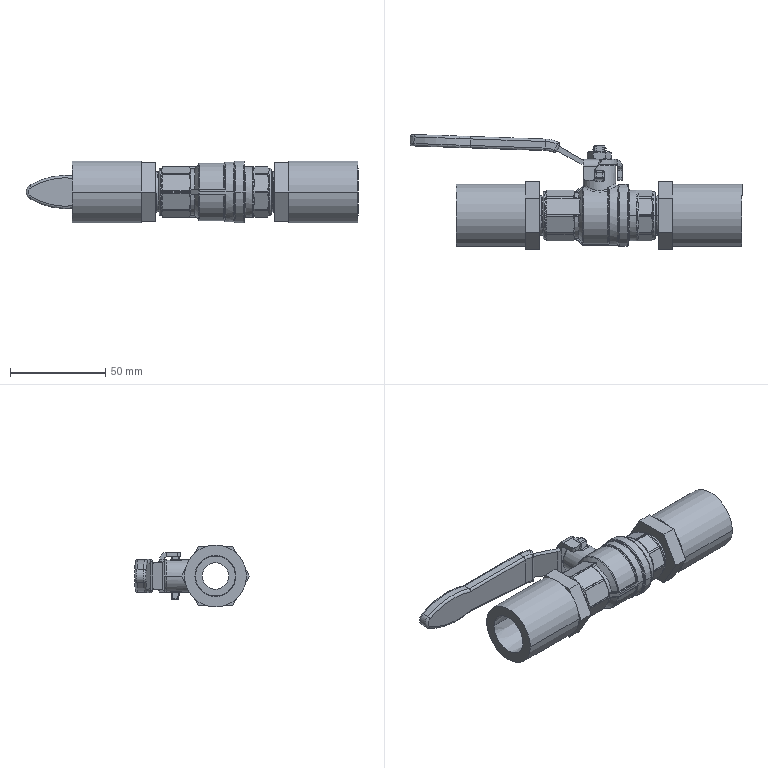Part | SolidWorks | 8 solids | 924 faces | box 174.317 x 60.383 x 32.544 mm | volume 89512 mm3 | spline 267 | plane 211 | cylinder 186 | cone 165 | sphere 52 | torus 43 | commonest cylinder face diameters 0.635 x62 7 x27 1.27 x20 2.54 x17 13.868 x8 0.254 x6